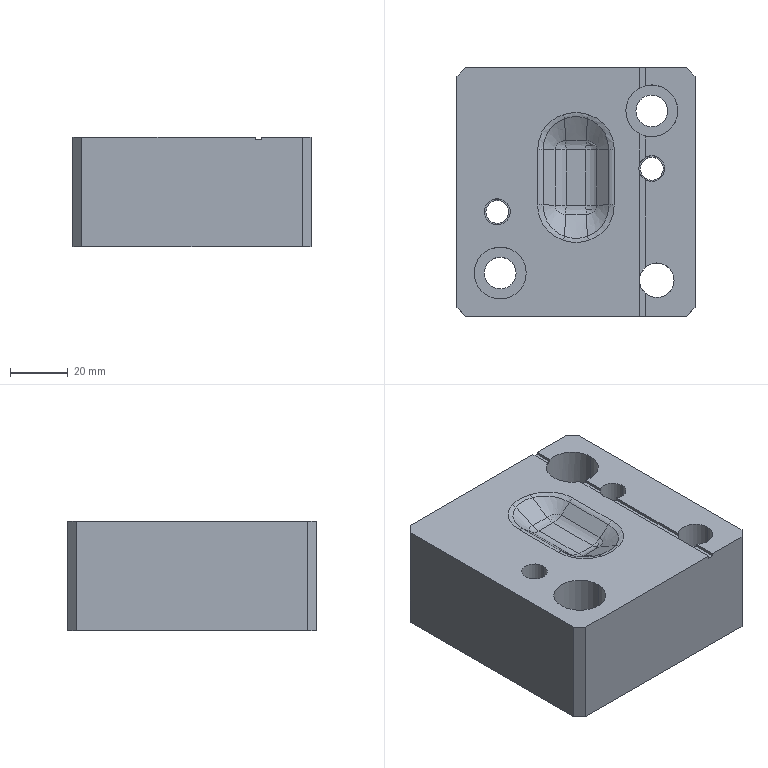Part | STEP file | 1_id998_x_t | 1 solid | 73 faces | box 82.5 x 86.2 x 38.01 mm | volume 245705 mm3 | plane 29 | cylinder 22 | spline 18 | cone 4 | commonest cylinder face diameters 7.938 x4 9 x4 11 x4 12 x4 18 x4 6 x2